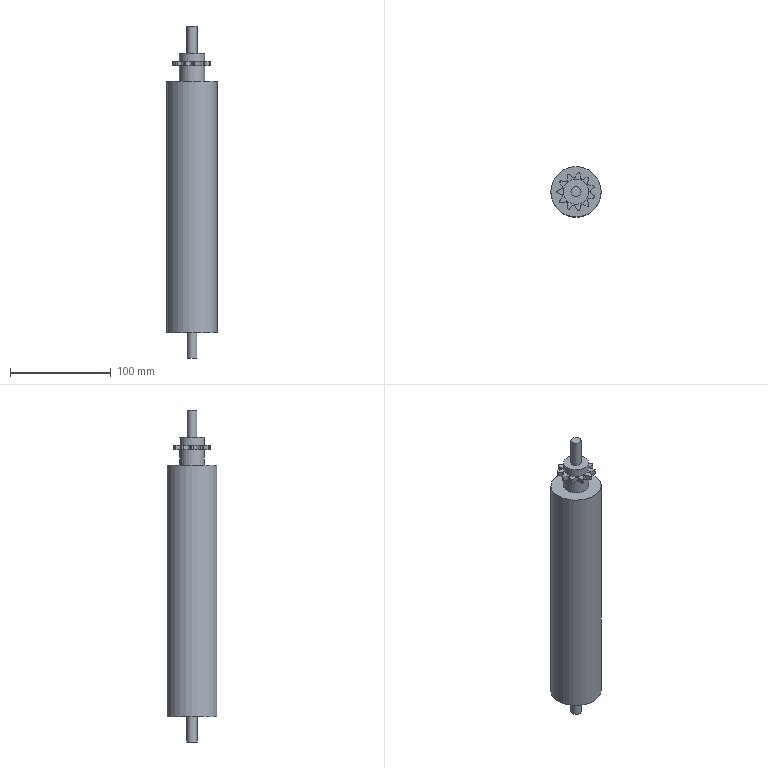Part | NX | 1 solid | 67 faces | box 50 x 50 x 330 mm | volume 510150 mm3 | cylinder 38 | plane 29 | commonest cylinder face diameters 3 x33 10 x2 25 x2 50 x1